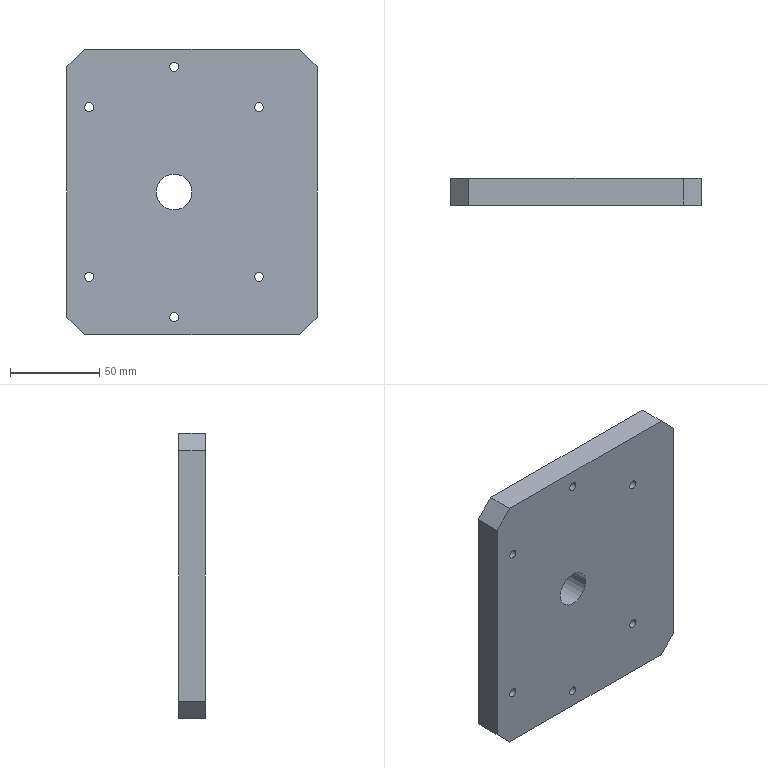Part | STEP file | Chamfer 1-24 | 1 solid | 24 faces | box 140 x 15 x 160 mm | volume 326520 mm3 | cylinder 14 | plane 10 | commonest cylinder face diameters 5 x12 20 x2
STEP:
#1=CARTESIAN_POINT('',(-1538.738,1679.264,2864.251));
#2=VERTEX_POINT('',#1);
#3=CARTESIAN_POINT('',(-1533.738,1679.264,2864.251));
#4=VERTEX_POINT('',#3);
#5=CARTESIAN_POINT('',(-1536.238,1679.264,2864.251));
#6=DIRECTION('',(0.,1.,0.));
#7=DIRECTION('',(1.,0.,0.));
#8=AXIS2_PLACEMENT_3D('',#5,#6,#7);
#9=CIRCLE('',#8,2.5);
#10=EDGE_CURVE('',#2,#4,#9,.T.);
#11=ORIENTED_EDGE('',*,*,#10,.F.);
#12=CARTESIAN_POINT('',(-1538.738,1694.264,2864.251));
#13=VERTEX_POINT('',#12);
#14=CARTESIAN_POINT('',(-1538.738,1694.264,2864.251));
#15=DIRECTION('',(0.,1.,0.));
#16=VECTOR('',#15,1000.);
#17=LINE('',#14,#16);
#18=EDGE_CURVE('',#2,#13,#17,.T.);
#19=ORIENTED_EDGE('',*,*,#18,.T.);
#20=CARTESIAN_POINT('',(-1533.738,1694.264,2864.251));
#21=VERTEX_POINT('',#20);
#22=CARTESIAN_POINT('',(-1536.238,1694.264,2864.251));
#23=DIRECTION('',(0.,1.,0.));
#24=DIRECTION('',(1.,0.,0.));
#25=AXIS2_PLACEMENT_3D('',#22,#23,#24);
#26=CIRCLE('',#25,2.5);
#27=EDGE_CURVE('',#13,#21,#26,.T.);
#28=ORIENTED_EDGE('',*,*,#27,.T.);
#29=CARTESIAN_POINT('',(-1533.738,1694.264,2864.251));
#30=DIRECTION('',(0.,1.,0.));
#31=VECTOR('',#30,1000.);
#32=LINE('',#29,#31);
#33=EDGE_CURVE('',#4,#21,#32,.T.);
#34=ORIENTED_EDGE('',*,*,#33,.F.);
#35=EDGE_LOOP('',(#11,#19,#28,#34));
#36=FACE_OUTER_BOUND('',#35,.T.);
#37=CARTESIAN_POINT('',(-1536.238,1694.264,2864.251));
#38=DIRECTION('',(0.,1.,0.));
#39=DIRECTION('',(-1.,0.,0.));
#40=AXIS2_PLACEMENT_3D('',#37,#38,#39);
#41=CYLINDRICAL_SURFACE('',#40,2.5);
#42=ADVANCED_FACE('',(#36),#41,.F.);
#43=CARTESIAN_POINT('',(-1491.238,1679.264,2886.751));
#44=VERTEX_POINT('',#43);
#45=CARTESIAN_POINT('',(-1486.238,1679.264,2886.751));
#46=VERTEX_POINT('',#45);
#47=CARTESIAN_POINT('',(-1488.738,1679.264,2886.751));
#48=DIRECTION('',(0.,1.,0.));
#49=DIRECTION('',(1.,0.,0.));
#50=AXIS2_PLACEMENT_3D('',#47,#48,#49);
#51=CIRCLE('',#50,2.5);
#52=EDGE_CURVE('',#44,#46,#51,.T.);
#53=ORIENTED_EDGE('',*,*,#52,.F.);
#54=CARTESIAN_POINT('',(-1491.238,1694.264,2886.751));
#55=VERTEX_POINT('',#54);
#56=CARTESIAN_POINT('',(-1491.238,1694.264,2886.751));
#57=DIRECTION('',(0.,1.,0.));
#58=VECTOR('',#57,1000.);
#59=LINE('',#56,#58);
#60=EDGE_CURVE('',#44,#55,#59,.T.);
#61=ORIENTED_EDGE('',*,*,#60,.T.);
#62=CARTESIAN_POINT('',(-1486.238,1694.264,2886.751));
#63=VERTEX_POINT('',#62);
#64=CARTESIAN_POINT('',(-1488.738,1694.264,2886.751));
#65=DIRECTION('',(0.,1.,0.));
#66=DIRECTION('',(1.,0.,0.));
#67=AXIS2_PLACEMENT_3D('',#64,#65,#66);
#68=CIRCLE('',#67,2.5);
#69=EDGE_CURVE('',#55,#63,#68,.T.);
#70=ORIENTED_EDGE('',*,*,#69,.T.);
#71=CARTESIAN_POINT('',(-1486.238,1694.264,2886.751));
#72=DIRECTION('',(0.,1.,0.));
#73=VECTOR('',#72,1000.);
#74=LINE('',#71,#73);
#75=EDGE_CURVE('',#46,#63,#74,.T.);
#76=ORIENTED_EDGE('',*,*,#75,.F.);
#77=EDGE_LOOP('',(#53,#61,#70,#76));
#78=FACE_OUTER_BOUND('',#77,.T.);
#79=CARTESIAN_POINT('',(-1488.738,1694.264,2886.751));
#80=DIRECTION('',(0.,1.,0.));
#81=DIRECTION('',(-1.,0.,0.));
#82=AXIS2_PLACEMENT_3D('',#79,#80,#81);
#83=CYLINDRICAL_SURFACE('',#82,2.5);
#84=ADVANCED_FACE('',(#78),#83,.F.);
#85=CARTESIAN_POINT('',(-1538.738,1679.264,2769.251));
#86=VERTEX_POINT('',#85);
#87=CARTESIAN_POINT('',(-1533.738,1679.264,2769.251));
#88=VERTEX_POINT('',#87);
#89=CARTESIAN_POINT('',(-1536.238,1679.264,2769.251));
#90=DIRECTION('',(0.,1.,0.));
#91=DIRECTION('',(1.,0.,0.));
#92=AXIS2_PLACEMENT_3D('',#89,#90,#91);
#93=CIRCLE('',#92,2.5);
#94=EDGE_CURVE('',#86,#88,#93,.T.);
#95=ORIENTED_EDGE('',*,*,#94,.F.);
#96=CARTESIAN_POINT('',(-1538.738,1694.264,2769.251));
#97=VERTEX_POINT('',#96);
#98=CARTESIAN_POINT('',(-1538.738,1694.264,2769.251));
#99=DIRECTION('',(0.,1.,0.));
#100=VECTOR('',#99,1000.);
#101=LINE('',#98,#100);
#102=EDGE_CURVE('',#86,#97,#101,.T.);
#103=ORIENTED_EDGE('',*,*,#102,.T.);
#104=CARTESIAN_POINT('',(-1533.738,1694.264,2769.251));
#105=VERTEX_POINT('',#104);
#106=CARTESIAN_POINT('',(-1536.238,1694.264,2769.251));
#107=DIRECTION('',(0.,1.,0.));
#108=DIRECTION('',(1.,0.,0.));
#109=AXIS2_PLACEMENT_3D('',#106,#107,#108);
#110=CIRCLE('',#109,2.5);
#111=EDGE_CURVE('',#97,#105,#110,.T.);
#112=ORIENTED_EDGE('',*,*,#111,.T.);
#113=CARTESIAN_POINT('',(-1533.738,1694.264,2769.251));
#114=DIRECTION('',(0.,1.,0.));
#115=VECTOR('',#114,1000.);
#116=LINE('',#113,#115);
#117=EDGE_CURVE('',#88,#105,#116,.T.);
#118=ORIENTED_EDGE('',*,*,#117,.F.);
#119=EDGE_LOOP('',(#95,#103,#112,#118));
#120=FACE_OUTER_BOUND('',#119,.T.);
#121=CARTESIAN_POINT('',(-1536.238,1694.264,2769.251));
#122=DIRECTION('',(0.,1.,0.));
#123=DIRECTION('',(-1.,0.,0.));
#124=AXIS2_PLACEMENT_3D('',#121,#122,#123);
#125=CYLINDRICAL_SURFACE('',#124,2.5);
#126=ADVANCED_FACE('',(#120),#125,.F.);
#127=CARTESIAN_POINT('',(-1491.238,1679.264,2746.751));
#128=VERTEX_POINT('',#127);
#129=CARTESIAN_POINT('',(-1486.238,1679.264,2746.751));
#130=VERTEX_POINT('',#129);
#131=CARTESIAN_POINT('',(-1488.738,1679.264,2746.751));
#132=DIRECTION('',(0.,1.,0.));
#133=DIRECTION('',(1.,0.,0.));
#134=AXIS2_PLACEMENT_3D('',#131,#132,#133);
#135=CIRCLE('',#134,2.5);
#136=EDGE_CURVE('',#128,#130,#135,.T.);
#137=ORIENTED_EDGE('',*,*,#136,.F.);
#138=CARTESIAN_POINT('',(-1491.238,1694.264,2746.751));
#139=VERTEX_POINT('',#138);
#140=CARTESIAN_POINT('',(-1491.238,1694.264,2746.751));
#141=DIRECTION('',(0.,1.,0.));
#142=VECTOR('',#141,1000.);
#143=LINE('',#140,#142);
#144=EDGE_CURVE('',#128,#139,#143,.T.);
#145=ORIENTED_EDGE('',*,*,#144,.T.);
#146=CARTESIAN_POINT('',(-1486.238,1694.264,2746.751));
#147=VERTEX_POINT('',#146);
#148=CARTESIAN_POINT('',(-1488.738,1694.264,2746.751));
#149=DIRECTION('',(0.,1.,0.));
#150=DIRECTION('',(1.,0.,0.));
#151=AXIS2_PLACEMENT_3D('',#148,#149,#150);
#152=CIRCLE('',#151,2.5);
#153=EDGE_CURVE('',#139,#147,#152,.T.);
#154=ORIENTED_EDGE('',*,*,#153,.T.);
#155=CARTESIAN_POINT('',(-1486.238,1694.264,2746.751));
#156=DIRECTION('',(0.,1.,0.));
#157=VECTOR('',#156,1000.);
#158=LINE('',#155,#157);
#159=EDGE_CURVE('',#130,#147,#158,.T.);
#160=ORIENTED_EDGE('',*,*,#159,.F.);
#161=EDGE_LOOP('',(#137,#145,#154,#160));
#162=FACE_OUTER_BOUND('',#161,.T.);
#163=CARTESIAN_POINT('',(-1488.738,1694.264,2746.751));
#164=DIRECTION('',(0.,1.,0.));
#165=DIRECTION('',(-1.,0.,0.));
#166=AXIS2_PLACEMENT_3D('',#163,#164,#165);
#167=CYLINDRICAL_SURFACE('',#166,2.5);
#168=ADVANCED_FACE('',(#162),#167,.F.);
#169=CARTESIAN_POINT('',(-1443.738,1679.264,2864.251));
#170=VERTEX_POINT('',#169);
#171=CARTESIAN_POINT('',(-1438.738,1679.264,2864.251));
#172=VERTEX_POINT('',#171);
#173=CARTESIAN_POINT('',(-1441.238,1679.264,2864.251));
#174=DIRECTION('',(0.,1.,0.));
#175=DIRECTION('',(1.,0.,0.));
#176=AXIS2_PLACEMENT_3D('',#173,#174,#175);
#177=CIRCLE('',#176,2.5);
#178=EDGE_CURVE('',#170,#172,#177,.T.);
#179=ORIENTED_EDGE('',*,*,#178,.F.);
#180=CARTESIAN_POINT('',(-1443.738,1694.264,2864.251));
#181=VERTEX_POINT('',#180);
#182=CARTESIAN_POINT('',(-1443.738,1694.264,2864.251));
#183=DIRECTION('',(0.,1.,0.));
#184=VECTOR('',#183,1000.);
#185=LINE('',#182,#184);
#186=EDGE_CURVE('',#170,#181,#185,.T.);
#187=ORIENTED_EDGE('',*,*,#186,.T.);
#188=CARTESIAN_POINT('',(-1438.738,1694.264,2864.251));
#189=VERTEX_POINT('',#188);
#190=CARTESIAN_POINT('',(-1441.238,1694.264,2864.251));
#191=DIRECTION('',(0.,1.,0.));
#192=DIRECTION('',(1.,0.,0.));
#193=AXIS2_PLACEMENT_3D('',#190,#191,#192);
#194=CIRCLE('',#193,2.5);
#195=EDGE_CURVE('',#181,#189,#194,.T.);
#196=ORIENTED_EDGE('',*,*,#195,.T.);
#197=CARTESIAN_POINT('',(-1438.738,1694.264,2864.251));
#198=DIRECTION('',(0.,1.,0.));
#199=VECTOR('',#198,1000.);
#200=LINE('',#197,#199);
#201=EDGE_CURVE('',#172,#189,#200,.T.);
#202=ORIENTED_EDGE('',*,*,#201,.F.);
#203=EDGE_LOOP('',(#179,#187,#196,#202));
#204=FACE_OUTER_BOUND('',#203,.T.);
#205=CARTESIAN_POINT('',(-1441.238,1694.264,2864.251));
#206=DIRECTION('',(0.,1.,0.));
#207=DIRECTION('',(-1.,0.,0.));
#208=AXIS2_PLACEMENT_3D('',#205,#206,#207);
#209=CYLINDRICAL_SURFACE('',#208,2.5);
#210=ADVANCED_FACE('',(#204),#209,.F.);
#211=CARTESIAN_POINT('',(-1443.738,1679.264,2769.251));
#212=VERTEX_POINT('',#211);
#213=CARTESIAN_POINT('',(-1438.738,1679.264,2769.251));
#214=VERTEX_POINT('',#213);
#215=CARTESIAN_POINT('',(-1441.238,1679.264,2769.251));
#216=DIRECTION('',(0.,1.,0.));
#217=DIRECTION('',(1.,0.,0.));
#218=AXIS2_PLACEMENT_3D('',#215,#216,#217);
#219=CIRCLE('',#218,2.5);
#220=EDGE_CURVE('',#212,#214,#219,.T.);
#221=ORIENTED_EDGE('',*,*,#220,.F.);
#222=CARTESIAN_POINT('',(-1443.738,1694.264,2769.251));
#223=VERTEX_POINT('',#222);
#224=CARTESIAN_POINT('',(-1443.738,1694.264,2769.251));
#225=DIRECTION('',(0.,1.,0.));
#226=VECTOR('',#225,1000.);
#227=LINE('',#224,#226);
#228=EDGE_CURVE('',#212,#223,#227,.T.);
#229=ORIENTED_EDGE('',*,*,#228,.T.);
#230=CARTESIAN_POINT('',(-1438.738,1694.264,2769.251));
#231=VERTEX_POINT('',#230);
#232=CARTESIAN_POINT('',(-1441.238,1694.264,2769.251));
#233=DIRECTION('',(0.,1.,0.));
#234=DIRECTION('',(1.,0.,0.));
#235=AXIS2_PLACEMENT_3D('',#232,#233,#234);
#236=CIRCLE('',#235,2.5);
#237=EDGE_CURVE('',#223,#231,#236,.T.);
#238=ORIENTED_EDGE('',*,*,#237,.T.);
#239=CARTESIAN_POINT('',(-1438.738,1694.264,2769.251));
#240=DIRECTION('',(0.,1.,0.));
#241=VECTOR('',#240,1000.);
#242=LINE('',#239,#241);
#243=EDGE_CURVE('',#214,#231,#242,.T.);
#244=ORIENTED_EDGE('',*,*,#243,.F.);
#245=EDGE_LOOP('',(#221,#229,#238,#244));
#246=FACE_OUTER_BOUND('',#245,.T.);
#247=CARTESIAN_POINT('',(-1441.238,1694.264,2769.251));
#248=DIRECTION('',(0.,1.,0.));
#249=DIRECTION('',(-1.,0.,0.));
#250=AXIS2_PLACEMENT_3D('',#247,#248,#249);
#251=CYLINDRICAL_SURFACE('',#250,2.5);
#252=ADVANCED_FACE('',(#246),#251,.F.);
#253=CARTESIAN_POINT('',(-1498.738,1679.264,2816.751));
#254=VERTEX_POINT('',#253);
#255=CARTESIAN_POINT('',(-1478.738,1679.264,2816.751));
#256=VERTEX_POINT('',#255);
#257=CARTESIAN_POINT('',(-1488.738,1679.264,2816.751));
#258=DIRECTION('',(0.,1.,0.));
#259=DIRECTION('',(1.,0.,0.));
#260=AXIS2_PLACEMENT_3D('',#257,#258,#259);
#261=CIRCLE('',#260,10.);
#262=EDGE_CURVE('',#254,#256,#261,.T.);
#263=ORIENTED_EDGE('',*,*,#262,.F.);
#264=CARTESIAN_POINT('',(-1498.738,1694.264,2816.751));
#265=VERTEX_POINT('',#264);
#266=CARTESIAN_POINT('',(-1498.738,1634.264,2816.751));
#267=DIRECTION('',(0.,1.,0.));
#268=VECTOR('',#267,1000.);
#269=LINE('',#266,#268);
#270=EDGE_CURVE('',#254,#265,#269,.T.);
#271=ORIENTED_EDGE('',*,*,#270,.T.);
#272=CARTESIAN_POINT('',(-1478.738,1694.264,2816.751));
#273=VERTEX_POINT('',#272);
#274=CARTESIAN_POINT('',(-1488.738,1694.264,2816.751));
#275=DIRECTION('',(0.,1.,0.));
#276=DIRECTION('',(1.,0.,0.));
#277=AXIS2_PLACEMENT_3D('',#274,#275,#276);
#278=CIRCLE('',#277,10.);
#279=EDGE_CURVE('',#265,#273,#278,.T.);
#280=ORIENTED_EDGE('',*,*,#279,.T.);
#281=CARTESIAN_POINT('',(-1478.738,1634.264,2816.751));
#282=DIRECTION('',(0.,1.,0.));
#283=VECTOR('',#282,1000.);
#284=LINE('',#281,#283);
#285=EDGE_CURVE('',#256,#273,#284,.T.);
#286=ORIENTED_EDGE('',*,*,#285,.F.);
#287=EDGE_LOOP('',(#263,#271,#280,#286));
#288=FACE_OUTER_BOUND('',#287,.T.);
#289=CARTESIAN_POINT('',(-1488.738,1634.264,2816.751));
#290=DIRECTION('',(0.,1.,0.));
#291=DIRECTION('',(-1.,0.,0.));
#292=AXIS2_PLACEMENT_3D('',#289,#290,#291);
#293=CYLINDRICAL_SURFACE('',#292,10.);
#294=ADVANCED_FACE('',(#288),#293,.F.);
#295=CARTESIAN_POINT('',(-1418.738,1679.264,2736.751));
#296=VERTEX_POINT('',#295);
#297=CARTESIAN_POINT('',(-1538.738,1679.264,2736.751));
#298=VERTEX_POINT('',#297);
#299=CARTESIAN_POINT('',(-1548.738,1679.264,2736.751));
#300=DIRECTION('',(-1.,0.,0.));
#301=VECTOR('',#300,1000.);
#302=LINE('',#299,#301);
#303=EDGE_CURVE('',#296,#298,#302,.T.);
#304=ORIENTED_EDGE('',*,*,#303,.T.);
#305=CARTESIAN_POINT('',(-1538.738,1694.264,2736.751));
#306=VERTEX_POINT('',#305);
#307=CARTESIAN_POINT('',(-1538.738,1694.264,2736.751));
#308=DIRECTION('',(0.,1.,0.));
#309=VECTOR('',#308,1000.);
#310=LINE('',#307,#309);
#311=EDGE_CURVE('',#298,#306,#310,.T.);
#312=ORIENTED_EDGE('',*,*,#311,.T.);
#313=CARTESIAN_POINT('',(-1418.738,1694.264,2736.751));
#314=VERTEX_POINT('',#313);
#315=CARTESIAN_POINT('',(-1548.738,1694.264,2736.751));
#316=DIRECTION('',(-1.,0.,0.));
#317=VECTOR('',#316,1000.);
#318=LINE('',#315,#317);
#319=EDGE_CURVE('',#314,#306,#318,.T.);
#320=ORIENTED_EDGE('',*,*,#319,.F.);
#321=CARTESIAN_POINT('',(-1418.738,1694.264,2736.751));
#322=DIRECTION('',(0.,-1.,0.));
#323=VECTOR('',#322,1000.);
#324=LINE('',#321,#323);
#325=EDGE_CURVE('',#314,#296,#324,.T.);
#326=ORIENTED_EDGE('',*,*,#325,.T.);
#327=EDGE_LOOP('',(#304,#312,#320,#326));
#328=FACE_OUTER_BOUND('',#327,.T.);
#329=CARTESIAN_POINT('',(-1548.738,1694.264,2736.751));
#330=DIRECTION('',(0.,0.,1.));
#331=DIRECTION('',(-1.,0.,0.));
#332=AXIS2_PLACEMENT_3D('',#329,#330,#331);
#333=PLANE('',#332);
#334=ADVANCED_FACE('',(#328),#333,.F.);
#335=CARTESIAN_POINT('',(-1548.738,1694.264,2746.751));
#336=VERTEX_POINT('',#335);
#337=CARTESIAN_POINT('',(-1548.738,1694.264,2886.751));
#338=VERTEX_POINT('',#337);
#339=CARTESIAN_POINT('',(-1548.738,1694.264,2896.751));
#340=DIRECTION('',(0.,0.,1.));
#341=VECTOR('',#340,1000.);
#342=LINE('',#339,#341);
#343=EDGE_CURVE('',#336,#338,#342,.T.);
#344=ORIENTED_EDGE('',*,*,#343,.F.);
#345=CARTESIAN_POINT('',(-1548.738,1679.264,2746.751));
#346=VERTEX_POINT('',#345);
#347=CARTESIAN_POINT('',(-1548.738,1694.264,2746.751));
#348=DIRECTION('',(0.,-1.,0.));
#349=VECTOR('',#348,1000.);
#350=LINE('',#347,#349);
#351=EDGE_CURVE('',#336,#346,#350,.T.);
#352=ORIENTED_EDGE('',*,*,#351,.T.);
#353=CARTESIAN_POINT('',(-1548.738,1679.264,2886.751));
#354=VERTEX_POINT('',#353);
#355=CARTESIAN_POINT('',(-1548.738,1679.264,2896.751));
#356=DIRECTION('',(0.,0.,1.));
#357=VECTOR('',#356,1000.);
#358=LINE('',#355,#357);
#359=EDGE_CURVE('',#346,#354,#358,.T.);
#360=ORIENTED_EDGE('',*,*,#359,.T.);
#361=CARTESIAN_POINT('',(-1548.738,1694.264,2886.751));
#362=DIRECTION('',(0.,1.,0.));
#363=VECTOR('',#362,1000.);
#364=LINE('',#361,#363);
#365=EDGE_CURVE('',#354,#338,#364,.T.);
#366=ORIENTED_EDGE('',*,*,#365,.T.);
#367=EDGE_LOOP('',(#344,#352,#360,#366));
#368=FACE_OUTER_BOUND('',#367,.T.);
#369=CARTESIAN_POINT('',(-1548.738,1694.264,2896.751));
#370=DIRECTION('',(1.,0.,0.));
#371=DIRECTION('',(0.,0.,1.));
#372=AXIS2_PLACEMENT_3D('',#369,#370,#371);
#373=PLANE('',#372);
#374=ADVANCED_FACE('',(#368),#373,.F.);
#375=CARTESIAN_POINT('',(-1538.738,1679.264,2896.751));
#376=VERTEX_POINT('',#375);
#377=CARTESIAN_POINT('',(-1418.738,1679.264,2896.751));
#378=VERTEX_POINT('',#377);
#379=CARTESIAN_POINT('',(-1548.738,1679.264,2896.751));
#380=DIRECTION('',(1.,0.,0.));
#381=VECTOR('',#380,1000.);
#382=LINE('',#379,#381);
#383=EDGE_CURVE('',#376,#378,#382,.T.);
#384=ORIENTED_EDGE('',*,*,#383,.T.);
#385=CARTESIAN_POINT('',(-1418.738,1694.264,2896.751));
#386=VERTEX_POINT('',#385);
#387=CARTESIAN_POINT('',(-1418.738,1694.264,2896.751));
#388=DIRECTION('',(0.,1.,0.));
#389=VECTOR('',#388,1000.);
#390=LINE('',#387,#389);
#391=EDGE_CURVE('',#378,#386,#390,.T.);
#392=ORIENTED_EDGE('',*,*,#391,.T.);
#393=CARTESIAN_POINT('',(-1538.738,1694.264,2896.751));
#394=VERTEX_POINT('',#393);
#395=CARTESIAN_POINT('',(-1548.738,1694.264,2896.751));
#396=DIRECTION('',(1.,0.,0.));
#397=VECTOR('',#396,1000.);
#398=LINE('',#395,#397);
#399=EDGE_CURVE('',#394,#386,#398,.T.);
#400=ORIENTED_EDGE('',*,*,#399,.F.);
#401=CARTESIAN_POINT('',(-1538.738,1694.264,2896.751));
#402=DIRECTION('',(0.,-1.,0.));
#403=VECTOR('',#402,1000.);
#404=LINE('',#401,#403);
#405=EDGE_CURVE('',#394,#376,#404,.T.);
#406=ORIENTED_EDGE('',*,*,#405,.T.);
#407=EDGE_LOOP('',(#384,#392,#400,#406));
#408=FACE_OUTER_BOUND('',#407,.T.);
#409=CARTESIAN_POINT('',(-1548.738,1694.264,2896.751));
#410=DIRECTION('',(0.,0.,-1.));
#411=DIRECTION('',(1.,0.,0.));
#412=AXIS2_PLACEMENT_3D('',#409,#410,#411);
#413=PLANE('',#412);
#414=ADVANCED_FACE('',(#408),#413,.F.);
#415=CARTESIAN_POINT('',(-1408.738,1679.264,2886.751));
#416=VERTEX_POINT('',#415);
#417=CARTESIAN_POINT('',(-1408.738,1679.264,2746.751));
#418=VERTEX_POINT('',#417);
#419=CARTESIAN_POINT('',(-1408.738,1679.264,2896.751));
#420=DIRECTION('',(0.,0.,-1.));
#421=VECTOR('',#420,1000.);
#422=LINE('',#419,#421);
#423=EDGE_CURVE('',#416,#418,#422,.T.);
#424=ORIENTED_EDGE('',*,*,#423,.T.);
#425=CARTESIAN_POINT('',(-1408.738,1694.264,2746.751));
#426=VERTEX_POINT('',#425);
#427=CARTESIAN_POINT('',(-1408.738,1694.264,2746.751));
#428=DIRECTION('',(0.,1.,0.));
#429=VECTOR('',#428,1000.);
#430=LINE('',#427,#429);
#431=EDGE_CURVE('',#418,#426,#430,.T.);
#432=ORIENTED_EDGE('',*,*,#431,.T.);
#433=CARTESIAN_POINT('',(-1408.738,1694.264,2886.751));
#434=VERTEX_POINT('',#433);
#435=CARTESIAN_POINT('',(-1408.738,1694.264,2896.751));
#436=DIRECTION('',(0.,0.,-1.));
#437=VECTOR('',#436,1000.);
#438=LINE('',#435,#437);
#439=EDGE_CURVE('',#434,#426,#438,.T.);
#440=ORIENTED_EDGE('',*,*,#439,.F.);
#441=CARTESIAN_POINT('',(-1408.738,1694.264,2886.751));
#442=DIRECTION('',(0.,-1.,0.));
#443=VECTOR('',#442,1000.);
#444=LINE('',#441,#443);
#445=EDGE_CURVE('',#434,#416,#444,.T.);
#446=ORIENTED_EDGE('',*,*,#445,.T.);
#447=EDGE_LOOP('',(#424,#432,#440,#446));
#448=FACE_OUTER_BOUND('',#447,.T.);
#449=CARTESIAN_POINT('',(-1408.738,1694.264,2896.751));
#450=DIRECTION('',(-1.,0.,0.));
#451=DIRECTION('',(0.,0.,-1.));
#452=AXIS2_PLACEMENT_3D('',#449,#450,#451);
#453=PLANE('',#452);
#454=ADVANCED_FACE('',(#448),#453,.F.);
#455=CARTESIAN_POINT('',(-1536.238,1694.264,2864.251));
#456=DIRECTION('',(0.,1.,0.));
#457=DIRECTION('',(1.,0.,0.));
#458=AXIS2_PLACEMENT_3D('',#455,#456,#457);
#459=CIRCLE('',#458,2.5);
#460=EDGE_CURVE('',#21,#13,#459,.T.);
#461=ORIENTED_EDGE('',*,*,#460,.F.);
#462=ORIENTED_EDGE('',*,*,#27,.F.);
#463=EDGE_LOOP('',(#461,#462));
#464=FACE_BOUND('',#463,.T.);
#465=CARTESIAN_POINT('',(-1488.738,1694.264,2886.751));
#466=DIRECTION('',(0.,1.,0.));
#467=DIRECTION('',(1.,0.,0.));
#468=AXIS2_PLACEMENT_3D('',#465,#466,#467);
#469=CIRCLE('',#468,2.5);
#470=EDGE_CURVE('',#63,#55,#469,.T.);
#471=ORIENTED_EDGE('',*,*,#470,.F.);
#472=ORIENTED_EDGE('',*,*,#69,.F.);
#473=EDGE_LOOP('',(#471,#472));
#474=FACE_BOUND('',#473,.T.);
#475=CARTESIAN_POINT('',(-1536.238,1694.264,2769.251));
#476=DIRECTION('',(0.,1.,0.));
#477=DIRECTION('',(1.,0.,0.));
#478=AXIS2_PLACEMENT_3D('',#475,#476,#477);
#479=CIRCLE('',#478,2.5);
#480=EDGE_CURVE('',#105,#97,#479,.T.);
#481=ORIENTED_EDGE('',*,*,#480,.F.);
#482=ORIENTED_EDGE('',*,*,#111,.F.);
#483=EDGE_LOOP('',(#481,#482));
#484=FACE_BOUND('',#483,.T.);
#485=CARTESIAN_POINT('',(-1488.738,1694.264,2746.751));
#486=DIRECTION('',(0.,1.,0.));
#487=DIRECTION('',(1.,0.,0.));
#488=AXIS2_PLACEMENT_3D('',#485,#486,#487);
#489=CIRCLE('',#488,2.5);
#490=EDGE_CURVE('',#147,#139,#489,.T.);
#491=ORIENTED_EDGE('',*,*,#490,.F.);
#492=ORIENTED_EDGE('',*,*,#153,.F.);
#493=EDGE_LOOP('',(#491,#492));
#494=FACE_BOUND('',#493,.T.);
#495=CARTESIAN_POINT('',(-1441.238,1694.264,2864.251));
#496=DIRECTION('',(0.,1.,0.));
#497=DIRECTION('',(1.,0.,0.));
#498=AXIS2_PLACEMENT_3D('',#495,#496,#497);
#499=CIRCLE('',#498,2.5);
#500=EDGE_CURVE('',#189,#181,#499,.T.);
#501=ORIENTED_EDGE('',*,*,#500,.F.);
#502=ORIENTED_EDGE('',*,*,#195,.F.);
#503=EDGE_LOOP('',(#501,#502));
#504=FACE_BOUND('',#503,.T.);
#505=CARTESIAN_POINT('',(-1441.238,1694.264,2769.251));
#506=DIRECTION('',(0.,1.,0.));
#507=DIRECTION('',(1.,0.,0.));
#508=AXIS2_PLACEMENT_3D('',#505,#506,#507);
#509=CIRCLE('',#508,2.5);
#510=EDGE_CURVE('',#231,#223,#509,.T.);
#511=ORIENTED_EDGE('',*,*,#510,.F.);
#512=ORIENTED_EDGE('',*,*,#237,.F.);
#513=EDGE_LOOP('',(#511,#512));
#514=FACE_BOUND('',#513,.T.);
#515=CARTESIAN_POINT('',(-1488.738,1694.264,2816.751));
#516=DIRECTION('',(0.,1.,0.));
#517=DIRECTION('',(1.,0.,0.));
#518=AXIS2_PLACEMENT_3D('',#515,#516,#517);
#519=CIRCLE('',#518,10.);
#520=EDGE_CURVE('',#273,#265,#519,.T.);
#521=ORIENTED_EDGE('',*,*,#520,.F.);
#522=ORIENTED_EDGE('',*,*,#279,.F.);
#523=EDGE_LOOP('',(#521,#522));
#524=FACE_BOUND('',#523,.T.);
#525=ORIENTED_EDGE('',*,*,#319,.T.);
#526=CARTESIAN_POINT('',(-1548.738,1694.264,2746.751));
#527=DIRECTION('',(-0.7071,0.,0.7071));
#528=VECTOR('',#527,1000.);
#529=LINE('',#526,#528);
#530=EDGE_CURVE('',#306,#336,#529,.T.);
#531=ORIENTED_EDGE('',*,*,#530,.T.);
#532=ORIENTED_EDGE('',*,*,#343,.T.);
#533=CARTESIAN_POINT('',(-1548.738,1694.264,2886.751));
#534=DIRECTION('',(0.7071,0.,0.7071));
#535=VECTOR('',#534,1000.);
#536=LINE('',#533,#535);
#537=EDGE_CURVE('',#338,#394,#536,.T.);
#538=ORIENTED_EDGE('',*,*,#537,.T.);
#539=ORIENTED_EDGE('',*,*,#399,.T.);
#540=CARTESIAN_POINT('',(-1408.738,1694.264,2886.751));
#541=DIRECTION('',(0.7071,0.,-0.7071));
#542=VECTOR('',#541,1000.);
#543=LINE('',#540,#542);
#544=EDGE_CURVE('',#386,#434,#543,.T.);
#545=ORIENTED_EDGE('',*,*,#544,.T.);
#546=ORIENTED_EDGE('',*,*,#439,.T.);
#547=CARTESIAN_POINT('',(-1408.738,1694.264,2746.751));
#548=DIRECTION('',(-0.7071,0.,-0.7071));
#549=VECTOR('',#548,1000.);
#550=LINE('',#547,#549);
#551=EDGE_CURVE('',#426,#314,#550,.T.);
#552=ORIENTED_EDGE('',*,*,#551,.T.);
#553=EDGE_LOOP('',(#525,#531,#532,#538,#539,#545,#546,#552));
#554=FACE_OUTER_BOUND('',#553,.T.);
#555=CARTESIAN_POINT('',(-1478.738,1694.264,2816.751));
#556=DIRECTION('',(0.,1.,0.));
#557=DIRECTION('',(-1.,0.,0.));
#558=AXIS2_PLACEMENT_3D('',#555,#556,#557);
#559=PLANE('',#558);
#560=ADVANCED_FACE('',(#464,#474,#484,#494,#504,#514,#524,#554),#559,.T.);
#561=CARTESIAN_POINT('',(-1536.238,1679.264,2864.251));
#562=DIRECTION('',(0.,1.,0.));
#563=DIRECTION('',(1.,0.,0.));
#564=AXIS2_PLACEMENT_3D('',#561,#562,#563);
#565=CIRCLE('',#564,2.5);
#566=EDGE_CURVE('',#4,#2,#565,.T.);
#567=ORIENTED_EDGE('',*,*,#566,.T.);
#568=ORIENTED_EDGE('',*,*,#10,.T.);
#569=EDGE_LOOP('',(#567,#568));
#570=FACE_BOUND('',#569,.T.);
#571=CARTESIAN_POINT('',(-1488.738,1679.264,2886.751));
#572=DIRECTION('',(0.,1.,0.));
#573=DIRECTION('',(1.,0.,0.));
#574=AXIS2_PLACEMENT_3D('',#571,#572,#573);
#575=CIRCLE('',#574,2.5);
#576=EDGE_CURVE('',#46,#44,#575,.T.);
#577=ORIENTED_EDGE('',*,*,#576,.T.);
#578=ORIENTED_EDGE('',*,*,#52,.T.);
#579=EDGE_LOOP('',(#577,#578));
#580=FACE_BOUND('',#579,.T.);
#581=CARTESIAN_POINT('',(-1536.238,1679.264,2769.251));
#582=DIRECTION('',(0.,1.,0.));
#583=DIRECTION('',(1.,0.,0.));
#584=AXIS2_PLACEMENT_3D('',#581,#582,#583);
#585=CIRCLE('',#584,2.5);
#586=EDGE_CURVE('',#88,#86,#585,.T.);
#587=ORIENTED_EDGE('',*,*,#586,.T.);
#588=ORIENTED_EDGE('',*,*,#94,.T.);
#589=EDGE_LOOP('',(#587,#588));
#590=FACE_BOUND('',#589,.T.);
#591=CARTESIAN_POINT('',(-1488.738,1679.264,2746.751));
#592=DIRECTION('',(0.,1.,0.));
#593=DIRECTION('',(1.,0.,0.));
#594=AXIS2_PLACEMENT_3D('',#591,#592,#593);
#595=CIRCLE('',#594,2.5);
#596=EDGE_CURVE('',#130,#128,#595,.T.);
#597=ORIENTED_EDGE('',*,*,#596,.T.);
#598=ORIENTED_EDGE('',*,*,#136,.T.);
#599=EDGE_LOOP('',(#597,#598));
#600=FACE_BOUND('',#599,.T.);
#601=CARTESIAN_POINT('',(-1441.238,1679.264,2864.251));
#602=DIRECTION('',(0.,1.,0.));
#603=DIRECTION('',(1.,0.,0.));
#604=AXIS2_PLACEMENT_3D('',#601,#602,#603);
#605=CIRCLE('',#604,2.5);
#606=EDGE_CURVE('',#172,#170,#605,.T.);
#607=ORIENTED_EDGE('',*,*,#606,.T.);
#608=ORIENTED_EDGE('',*,*,#178,.T.);
#609=EDGE_LOOP('',(#607,#608));
#610=FACE_BOUND('',#609,.T.);
#611=CARTESIAN_POINT('',(-1441.238,1679.264,2769.251));
#612=DIRECTION('',(0.,1.,0.));
#613=DIRECTION('',(1.,0.,0.));
#614=AXIS2_PLACEMENT_3D('',#611,#612,#613);
#615=CIRCLE('',#614,2.5);
#616=EDGE_CURVE('',#214,#212,#615,.T.);
#617=ORIENTED_EDGE('',*,*,#616,.T.);
#618=ORIENTED_EDGE('',*,*,#220,.T.);
#619=EDGE_LOOP('',(#617,#618));
#620=FACE_BOUND('',#619,.T.);
#621=CARTESIAN_POINT('',(-1488.738,1679.264,2816.751));
#622=DIRECTION('',(0.,1.,0.));
#623=DIRECTION('',(1.,0.,0.));
#624=AXIS2_PLACEMENT_3D('',#621,#622,#623);
#625=CIRCLE('',#624,10.);
#626=EDGE_CURVE('',#256,#254,#625,.T.);
#627=ORIENTED_EDGE('',*,*,#626,.T.);
#628=ORIENTED_EDGE('',*,*,#262,.T.);
#629=EDGE_LOOP('',(#627,#628));
#630=FACE_BOUND('',#629,.T.);
#631=ORIENTED_EDGE('',*,*,#359,.F.);
#632=CARTESIAN_POINT('',(-1548.738,1679.264,2746.751));
#633=DIRECTION('',(0.7071,0.,-0.7071));
#634=VECTOR('',#633,1000.);
#635=LINE('',#632,#634);
#636=EDGE_CURVE('',#346,#298,#635,.T.);
#637=ORIENTED_EDGE('',*,*,#636,.T.);
#638=ORIENTED_EDGE('',*,*,#303,.F.);
#639=CARTESIAN_POINT('',(-1418.738,1679.264,2736.751));
#640=DIRECTION('',(0.7071,0.,0.7071));
#641=VECTOR('',#640,1000.);
#642=LINE('',#639,#641);
#643=EDGE_CURVE('',#296,#418,#642,.T.);
#644=ORIENTED_EDGE('',*,*,#643,.T.);
#645=ORIENTED_EDGE('',*,*,#423,.F.);
#646=CARTESIAN_POINT('',(-1408.738,1679.264,2886.751));
#647=DIRECTION('',(-0.7071,0.,0.7071));
#648=VECTOR('',#647,1000.);
#649=LINE('',#646,#648);
#650=EDGE_CURVE('',#416,#378,#649,.T.);
#651=ORIENTED_EDGE('',*,*,#650,.T.);
#652=ORIENTED_EDGE('',*,*,#383,.F.);
#653=CARTESIAN_POINT('',(-1538.738,1679.264,2896.751));
#654=DIRECTION('',(-0.7071,0.,-0.7071));
#655=VECTOR('',#654,1000.);
#656=LINE('',#653,#655);
#657=EDGE_CURVE('',#376,#354,#656,.T.);
#658=ORIENTED_EDGE('',*,*,#657,.T.);
#659=EDGE_LOOP('',(#631,#637,#638,#644,#645,#651,#652,#658));
#660=FACE_OUTER_BOUND('',#659,.T.);
#661=CARTESIAN_POINT('',(-1478.738,1679.264,2816.751));
#662=DIRECTION('',(0.,1.,0.));
#663=DIRECTION('',(-1.,0.,0.));
#664=AXIS2_PLACEMENT_3D('',#661,#662,#663);
#665=PLANE('',#664);
#666=ADVANCED_FACE('',(#570,#580,#590,#600,#610,#620,#630,#660),#665,.F.);
#667=ORIENTED_EDGE('',*,*,#270,.F.);
#668=ORIENTED_EDGE('',*,*,#626,.F.);
#669=ORIENTED_EDGE('',*,*,#285,.T.);
#670=ORIENTED_EDGE('',*,*,#520,.T.);
#671=EDGE_LOOP('',(#667,#668,#669,#670));
#672=FACE_OUTER_BOUND('',#671,.T.);
#673=CARTESIAN_POINT('',(-1488.738,1634.264,2816.751));
#674=DIRECTION('',(0.,1.,0.));
#675=DIRECTION('',(-1.,0.,0.));
#676=AXIS2_PLACEMENT_3D('',#673,#674,#675);
#677=CYLINDRICAL_SURFACE('',#676,10.);
#678=ADVANCED_FACE('',(#672),#677,.F.);
#679=ORIENTED_EDGE('',*,*,#228,.F.);
#680=ORIENTED_EDGE('',*,*,#616,.F.);
#681=ORIENTED_EDGE('',*,*,#243,.T.);
#682=ORIENTED_EDGE('',*,*,#510,.T.);
#683=EDGE_LOOP('',(#679,#680,#681,#682));
#684=FACE_OUTER_BOUND('',#683,.T.);
#685=CARTESIAN_POINT('',(-1441.238,1694.264,2769.251));
#686=DIRECTION('',(0.,1.,0.));
#687=DIRECTION('',(-1.,0.,0.));
#688=AXIS2_PLACEMENT_3D('',#685,#686,#687);
#689=CYLINDRICAL_SURFACE('',#688,2.5);
#690=ADVANCED_FACE('',(#684),#689,.F.);
#691=ORIENTED_EDGE('',*,*,#186,.F.);
#692=ORIENTED_EDGE('',*,*,#606,.F.);
#693=ORIENTED_EDGE('',*,*,#201,.T.);
#694=ORIENTED_EDGE('',*,*,#500,.T.);
#695=EDGE_LOOP('',(#691,#692,#693,#694));
#696=FACE_OUTER_BOUND('',#695,.T.);
#697=CARTESIAN_POINT('',(-1441.238,1694.264,2864.251));
#698=DIRECTION('',(0.,1.,0.));
#699=DIRECTION('',(-1.,0.,0.));
#700=AXIS2_PLACEMENT_3D('',#697,#698,#699);
#701=CYLINDRICAL_SURFACE('',#700,2.5);
#702=ADVANCED_FACE('',(#696),#701,.F.);
#703=ORIENTED_EDGE('',*,*,#144,.F.);
#704=ORIENTED_EDGE('',*,*,#596,.F.);
#705=ORIENTED_EDGE('',*,*,#159,.T.);
#706=ORIENTED_EDGE('',*,*,#490,.T.);
#707=EDGE_LOOP('',(#703,#704,#705,#706));
#708=FACE_OUTER_BOUND('',#707,.T.);
#709=CARTESIAN_POINT('',(-1488.738,1694.264,2746.751));
#710=DIRECTION('',(0.,1.,0.));
#711=DIRECTION('',(-1.,0.,0.));
#712=AXIS2_PLACEMENT_3D('',#709,#710,#711);
#713=CYLINDRICAL_SURFACE('',#712,2.5);
#714=ADVANCED_FACE('',(#708),#713,.F.);
#715=ORIENTED_EDGE('',*,*,#102,.F.);
#716=ORIENTED_EDGE('',*,*,#586,.F.);
#717=ORIENTED_EDGE('',*,*,#117,.T.);
#718=ORIENTED_EDGE('',*,*,#480,.T.);
#719=EDGE_LOOP('',(#715,#716,#717,#718));
#720=FACE_OUTER_BOUND('',#719,.T.);
#721=CARTESIAN_POINT('',(-1536.238,1694.264,2769.251));
#722=DIRECTION('',(0.,1.,0.));
#723=DIRECTION('',(-1.,0.,0.));
#724=AXIS2_PLACEMENT_3D('',#721,#722,#723);
#725=CYLINDRICAL_SURFACE('',#724,2.5);
#726=ADVANCED_FACE('',(#720),#725,.F.);
#727=ORIENTED_EDGE('',*,*,#60,.F.);
#728=ORIENTED_EDGE('',*,*,#576,.F.);
#729=ORIENTED_EDGE('',*,*,#75,.T.);
#730=ORIENTED_EDGE('',*,*,#470,.T.);
#731=EDGE_LOOP('',(#727,#728,#729,#730));
#732=FACE_OUTER_BOUND('',#731,.T.);
#733=CARTESIAN_POINT('',(-1488.738,1694.264,2886.751));
#734=DIRECTION('',(0.,1.,0.));
#735=DIRECTION('',(-1.,0.,0.));
#736=AXIS2_PLACEMENT_3D('',#733,#734,#735);
#737=CYLINDRICAL_SURFACE('',#736,2.5);
#738=ADVANCED_FACE('',(#732),#737,.F.);
#739=ORIENTED_EDGE('',*,*,#18,.F.);
#740=ORIENTED_EDGE('',*,*,#566,.F.);
#741=ORIENTED_EDGE('',*,*,#33,.T.);
#742=ORIENTED_EDGE('',*,*,#460,.T.);
#743=EDGE_LOOP('',(#739,#740,#741,#742));
#744=FACE_OUTER_BOUND('',#743,.T.);
#745=CARTESIAN_POINT('',(-1536.238,1694.264,2864.251));
#746=DIRECTION('',(0.,1.,0.));
#747=DIRECTION('',(-1.,0.,0.));
#748=AXIS2_PLACEMENT_3D('',#745,#746,#747);
#749=CYLINDRICAL_SURFACE('',#748,2.5);
#750=ADVANCED_FACE('',(#744),#749,.F.);
#751=ORIENTED_EDGE('',*,*,#530,.F.);
#752=ORIENTED_EDGE('',*,*,#311,.F.);
#753=ORIENTED_EDGE('',*,*,#636,.F.);
#754=ORIENTED_EDGE('',*,*,#351,.F.);
#755=EDGE_LOOP('',(#751,#752,#753,#754));
#756=FACE_OUTER_BOUND('',#755,.T.);
#757=CARTESIAN_POINT('',(-1548.738,1694.264,2746.751));
#758=DIRECTION('',(0.7071,0.,0.7071));
#759=DIRECTION('',(0.,1.,0.));
#760=AXIS2_PLACEMENT_3D('',#757,#758,#759);
#761=PLANE('',#760);
#762=ADVANCED_FACE('',(#756),#761,.F.);
#763=ORIENTED_EDGE('',*,*,#551,.F.);
#764=ORIENTED_EDGE('',*,*,#431,.F.);
#765=ORIENTED_EDGE('',*,*,#643,.F.);
#766=ORIENTED_EDGE('',*,*,#325,.F.);
#767=EDGE_LOOP('',(#763,#764,#765,#766));
#768=FACE_OUTER_BOUND('',#767,.T.);
#769=CARTESIAN_POINT('',(-1418.738,1694.264,2736.751));
#770=DIRECTION('',(-0.7071,0.,0.7071));
#771=DIRECTION('',(0.,1.,0.));
#772=AXIS2_PLACEMENT_3D('',#769,#770,#771);
#773=PLANE('',#772);
#774=ADVANCED_FACE('',(#768),#773,.F.);
#775=ORIENTED_EDGE('',*,*,#544,.F.);
#776=ORIENTED_EDGE('',*,*,#391,.F.);
#777=ORIENTED_EDGE('',*,*,#650,.F.);
#778=ORIENTED_EDGE('',*,*,#445,.F.);
#779=EDGE_LOOP('',(#775,#776,#777,#778));
#780=FACE_OUTER_BOUND('',#779,.T.);
#781=CARTESIAN_POINT('',(-1408.738,1694.264,2886.751));
#782=DIRECTION('',(-0.7071,0.,-0.7071));
#783=DIRECTION('',(0.,1.,0.));
#784=AXIS2_PLACEMENT_3D('',#781,#782,#783);
#785=PLANE('',#784);
#786=ADVANCED_FACE('',(#780),#785,.F.);
#787=ORIENTED_EDGE('',*,*,#537,.F.);
#788=ORIENTED_EDGE('',*,*,#365,.F.);
#789=ORIENTED_EDGE('',*,*,#657,.F.);
#790=ORIENTED_EDGE('',*,*,#405,.F.);
#791=EDGE_LOOP('',(#787,#788,#789,#790));
#792=FACE_OUTER_BOUND('',#791,.T.);
#793=CARTESIAN_POINT('',(-1538.738,1694.264,2896.751));
#794=DIRECTION('',(0.7071,0.,-0.7071));
#795=DIRECTION('',(0.,1.,0.));
#796=AXIS2_PLACEMENT_3D('',#793,#794,#795);
#797=PLANE('',#796);
#798=ADVANCED_FACE('',(#792),#797,.F.);
#799=CLOSED_SHELL('',(#42,#84,#126,#168,#210,#252,#294,#334,#374,#414,#454,#560,#666,#678,#690,#702,#714,#726,#738,#750,#762,#774,#786,#798));
#800=MANIFOLD_SOLID_BREP('',#799);
#801=CARTESIAN_POINT('',(0.,0.,0.));
#802=DIRECTION('',(0.,0.,1.));
#803=DIRECTION('',(1.,0.,0.));
#804=AXIS2_PLACEMENT_3D('',#801,#802,#803);
#805=(LENGTH_UNIT()NAMED_UNIT(*)SI_UNIT(.MILLI.,.METRE.));
#806=UNCERTAINTY_MEASURE_WITH_UNIT(LENGTH_MEASURE(0.00001),#805,'','');
#807=(NAMED_UNIT(*)PLANE_ANGLE_UNIT()SI_UNIT($,.RADIAN.));
#808=(NAMED_UNIT(*)SI_UNIT($,.STERADIAN.)SOLID_ANGLE_UNIT());
#809=(GEOMETRIC_REPRESENTATION_CONTEXT(3)GLOBAL_UNCERTAINTY_ASSIGNED_CONTEXT((#806))GLOBAL_UNIT_ASSIGNED_CONTEXT((#805,#807,#808))REPRESENTATION_CONTEXT('',''));
#810=ADVANCED_BREP_SHAPE_REPRESENTATION('',(#800,#804),#809);